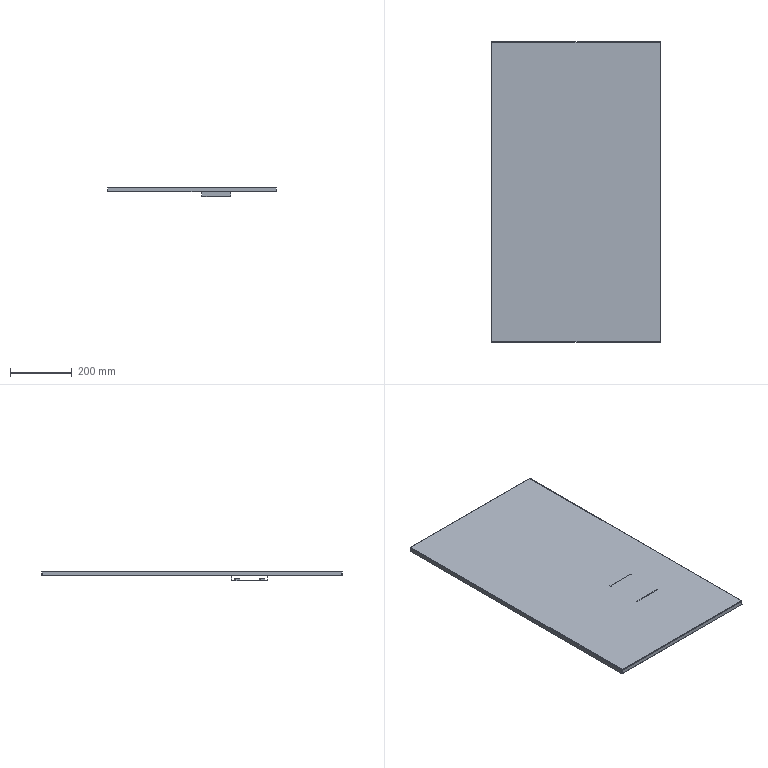Part | SolidWorks | features FlatPattern 2, SMBaseFlange 2, SheetMetal 2, HoleWzd 1, ICE 1, SMMiteredFlange 1 | 6 solids | 124 faces | box 550 x 973 x 31.5 mm | volume 890444 mm3 | plane 84 | cylinder 32 | spline 8 | commonest cylinder face diameters 5 x16 1.473 x8 4.473 x8